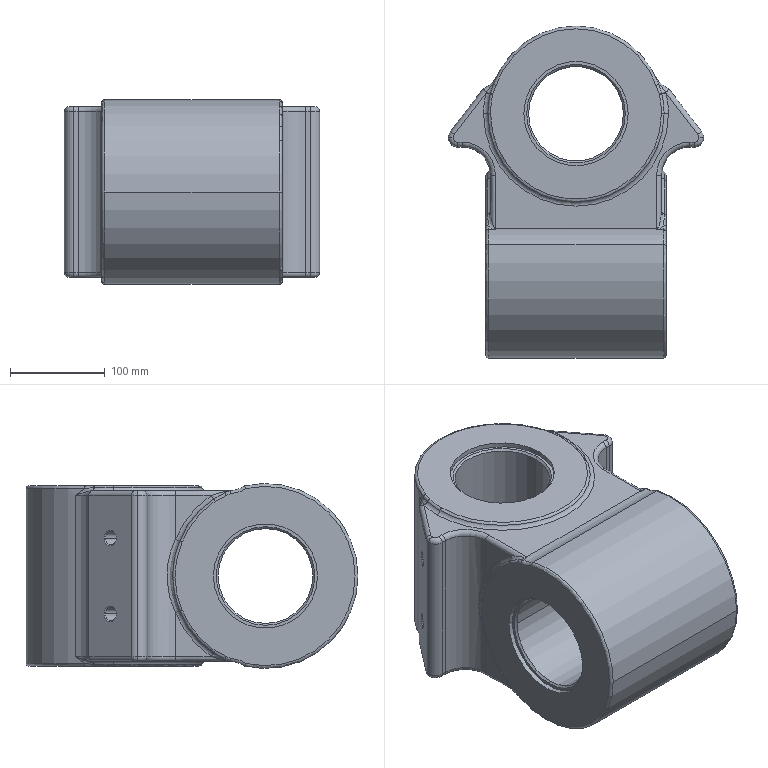Part | SolidWorks | features Fillet 12, ICE 10, MirrorPattern 3, Chamfer 2, 3DProfileFeature 1, Extrusion 1, HoleWzd 1 | 1 solid | 175 faces | box 269.383 x 350 x 195 mm | volume 8603541 mm3 | torus 53 | cylinder 48 | spline 32 | cone 24 | plane 18 | commonest cylinder face diameters 10 x12 14 x8 110 x8 60 x6 195 x6 100 x4